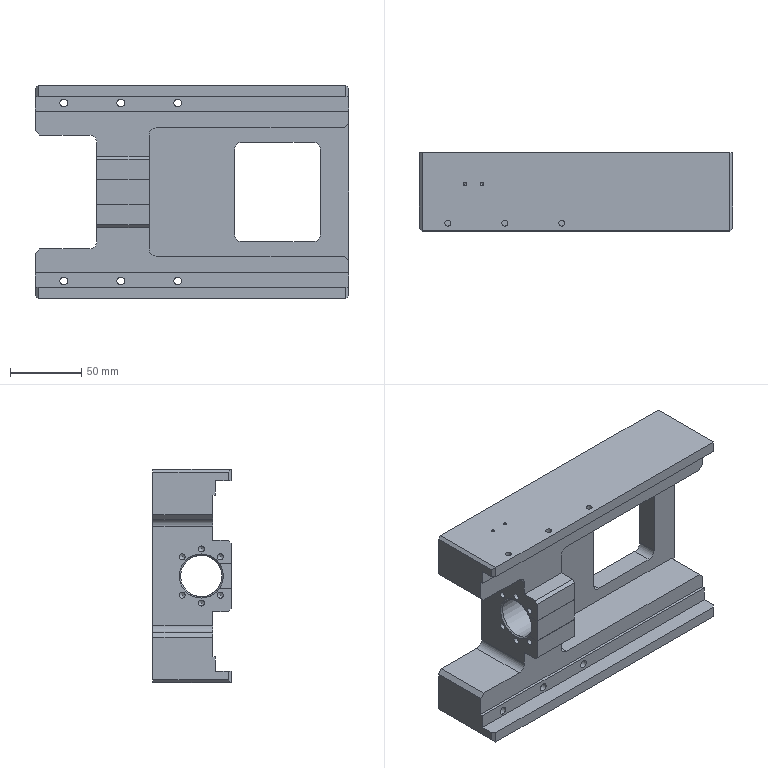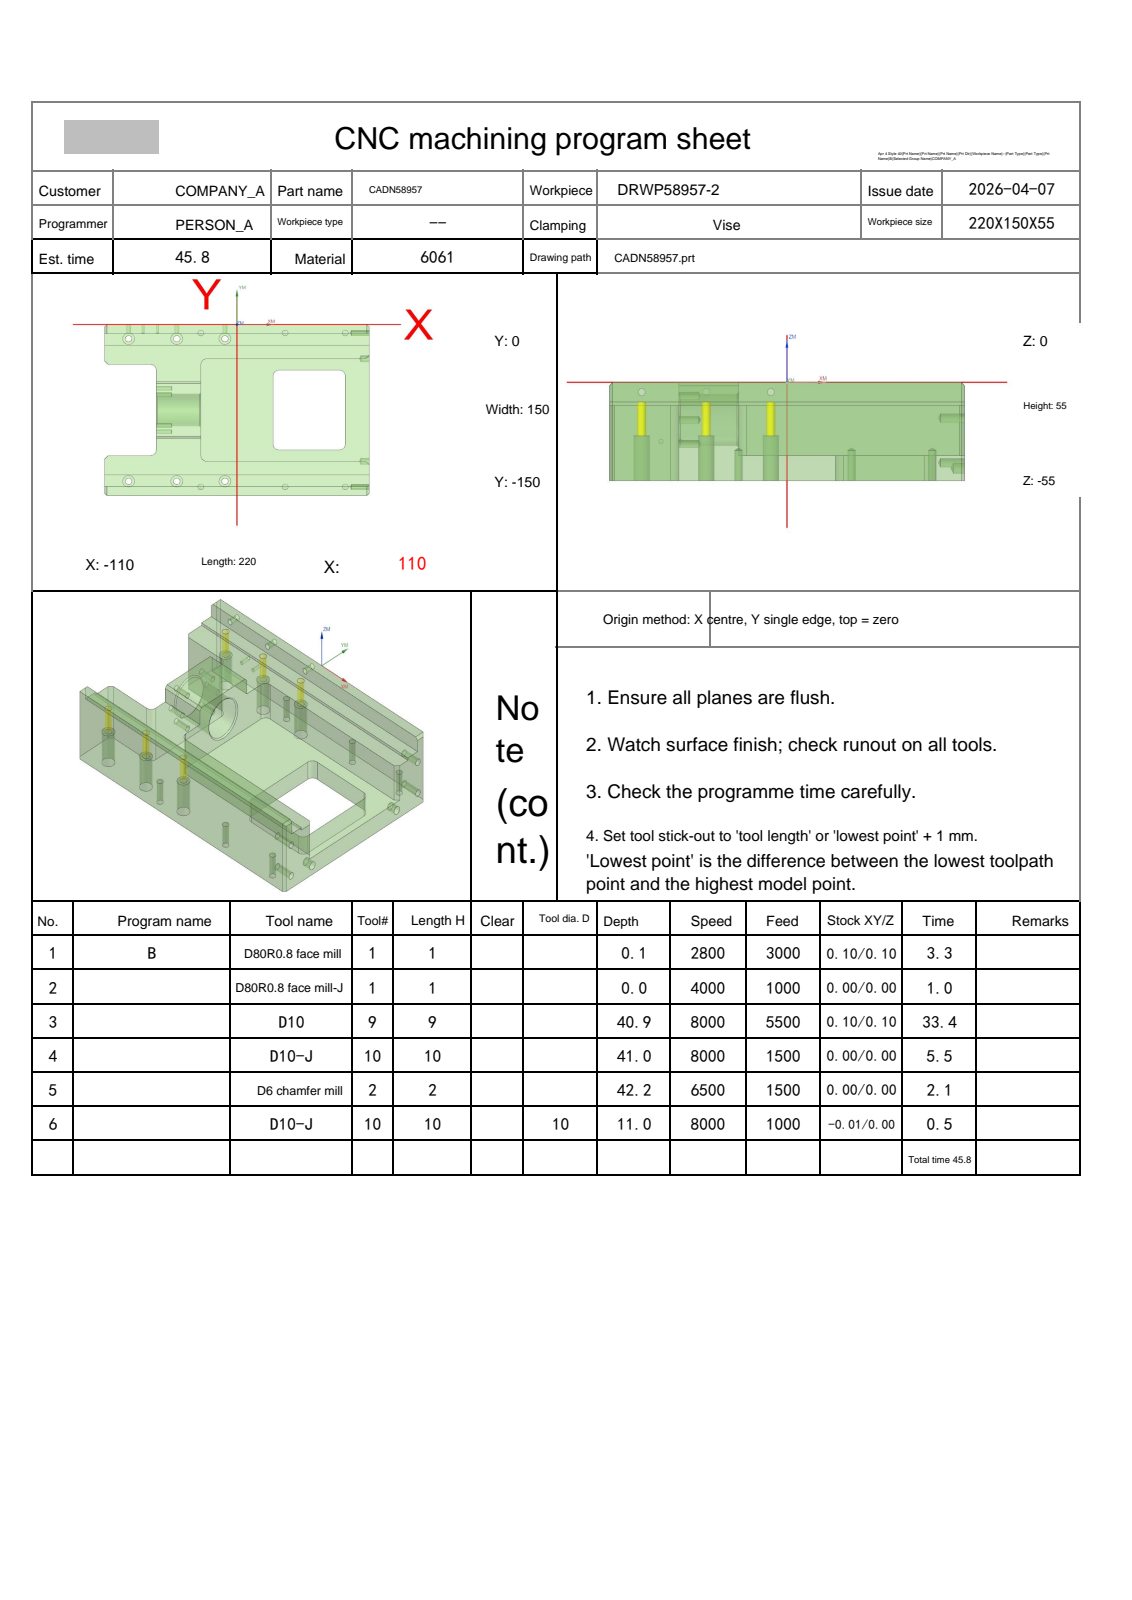NC program | NX | posted by the shop | part box 220 x 55 x 150 mm
Lines 14726 to 15484 of 15484:
N4 T10 M06
(D10-J  D=10. R=0. H=10 ce=0.40 di=0.00)
G00 G90 G54 X-117. Y-128.801 M03 S7000
G43 H10 Z14.5
M08
Z-9.5
G01 Z-11. F1500.
G03 X-115. Y-130.8 I2. J.001
G01 X114.1
G02 X115. Y-131.7 I0.0 J-.9
G01 Y-132.7
G02 X114. Y-133.7 I-1. J0.0
G01 X-114.1
G03 X-115. Y-134.6 I0.0 J-.9
G01 Y-135.6
G03 X-114. Y-136.6 I1. J0.0
G01 X115.
G03 X117. Y-134.6 I0.0 J2.
G01 Z-9.5
G00 Z14.5
Y-124.399
Z-11.5
G01 Z-13.
X113.
G03 X115. Y-126.399 I2. J0.0
G01 X-114.1
G02 X-115. Y-125.499 I0.0 J.9
G01 Y-123.199
G02 X-114. Y-122.199 I1. J0.0
G01 X114.201
G03 X115. Y-121.4 I-.001 J.8
G01 Y-121.343
G03 X114.707 Y-120.636 I-1. J0.0
G01 X112.363 Y-118.292
G03 X111.657 Y-117.999 I-.706 J-.708
G01 X-114.001
G02 X-115. Y-117. I.001 J1.
G01 Y-116.343
G02 X-114.707 Y-115.636 I1. J0.0
G01 X-113.163 Y-114.092
G02 X-112.457 Y-113.8 I.707 J-.708
G01 X-25.9
G03 X-25. Y-112.9 I0.0 J.9
G01 Y-110.6
G03 X-26. Y-109.6 I-1. J0.0
G01 X-71.1
G02 X-72. Y-108.7 I0.0 J.9
G01 Y-106.4
G02 X-71. Y-105.4 I1. J0.0
G01 X-25.
G02 X-23. Y-107.4 I0.0 J-2.
G01 Z-11.5
G00 Z14.5
Y-42.599
Z-11.5
G01 Z-13.
X-27.
G03 X-25. Y-44.599 I2. J0.0
G01 X-71.1
G02 X-72. Y-43.699 I0.0 J.9
G01 Y-41.399
G02 X-71. Y-40.399 I1. J0.0
G01 X-25.9
G03 X-25. Y-39.499 I0.0 J.9
G01 Y-37.199
G03 X-26. Y-36.199 I-1. J0.0
G01 X-112.458
G02 X-113.164 Y-35.907 I.001 J1.
G01 X-114.707 Y-34.364
G02 X-115. Y-33.657 I.707 J.707
G01 Y-32.999
G02 X-114.001 Y-32. I1. J-.001
G01 X111.658
G03 X112.364 Y-31.707 I-.001 J1.
G01 X114.707 Y-29.364
G03 X115. Y-28.657 I-.707 J.707
G01 Y-28.599
G03 X114.201 Y-27.8 I-.8 J-.001
G01 X-114.1
G02 X-115. Y-26.9 I0.0 J.9
G01 Y-24.6
G02 X-114. Y-23.6 I1. J0.0
G01 X115.
G02 X117. Y-25.6 I0.0 J-2.
G01 Z-11.5
G00 Z14.5
Y-21.199
Z-9.5
G01 Z-11.
G03 X115. Y-19.2 I-2. J-.001
G01 X-114.001
G02 X-115. Y-18.201 I.001 J1.
G01 Y-17.299
G02 X-114.001 Y-16.3 I1. J-.001
G01 X114.1
G03 X115. Y-15.4 I0.0 J.9
G01 Y-14.4
G03 X114. Y-13.4 I-1. J0.0
G01 X-115.
G03 X-117. Y-15.4 I0.0 J-2.
G01 Z-9.5
G00 Z14.5
G00 G90 X117. Y-73. M03 S7000
Z14.5
Z-39.5
G01 Z-41. F1500.
X113.
G03 X111. Y-75. I0.0 J-2.
G01 Y-115.882
G02 X110.8 Y-116.08 I-.2 J.001
G01 X110.66 Y-116.023
X109.237 Y-114.6
X-23.603
G02 X-24.6 Y-113.603 I.003 J1.
G01 Y-36.397
G02 X-23.603 Y-35.4 I1. J-.003
G01 X109.237
X110.66 Y-33.977
X110.8 Y-33.92
G02 X111. Y-34.118 I0.0 J-.2
G01 Y-77.086
G02 X110.707 Y-77.793 I-1. J0.0
G01 X106.293 Y-82.207
G03 X106. Y-82.914 I.707 J-.707
G01 Y-108.604
G02 X105.004 Y-109.6 I-1. J.004
G01 X-18.604
G02 X-19.6 Y-108.604 I.004 J1.
G01 Y-41.396
G02 X-18.604 Y-40.4 I1. J-.004
G01 X105.004
G02 X106. Y-41.396 I-.004 J-1.
G01 Y-77.086
G02 X105.707 Y-77.793 I-1. J0.0
G01 X101.293 Y-82.207
G03 X101. Y-82.914 I.707 J-.707
G01 Y-103.604
G02 X100.004 Y-104.6 I-1. J.004
G01 X-13.604
G02 X-14.6 Y-103.604 I.004 J1.
G01 Y-46.396
G02 X-13.604 Y-45.4 I1. J-.004
G01 X100.004
G02 X101. Y-46.396 I-.004 J-1.
G01 Y-77.086
G02 X100.707 Y-77.793 I-1. J0.0
G01 X96.293 Y-82.207
G03 X96. Y-82.914 I.707 J-.707
G01 Y-98.604
G02 X95.004 Y-99.6 I-1. J.004
G01 X-8.604
G02 X-9.6 Y-98.604 I.004 J1.
G01 Y-51.396
G02 X-8.604 Y-50.4 I1. J-.004
G01 X95.004
G02 X96. Y-51.396 I-.004 J-1.
G01 Y-77.086
G02 X95.707 Y-77.793 I-1. J0.0
G01 X91.293 Y-82.207
G03 X91. Y-82.914 I.707 J-.707
G01 Y-93.605
G02 X90.005 Y-94.6 I-1. J.005
G01 X-3.605
G02 X-4.6 Y-93.605 I.005 J1.
G01 Y-56.395
G02 X-3.605 Y-55.4 I1. J-.005
G01 X90.005
G02 X91. Y-56.395 I-.005 J-1.
G01 Y-77.086
G02 X90.707 Y-77.793 I-1. J0.0
G01 X86.293 Y-82.207
G03 X86. Y-82.914 I.707 J-.707
G01 Y-88.605
G02 X85.005 Y-89.6 I-1. J.005
G01 X1.395
G02 X.4 Y-88.605 I.005 J1.
G01 Y-61.395
G02 X1.395 Y-60.4 I1. J-.005
G01 X85.005
G02 X86. Y-61.395 I-.005 J-1.
G01 Y-77.086
G02 X85.707 Y-77.793 I-1. J0.0
G01 X81.292 Y-82.208
G03 X81. Y-82.914 I.708 J-.707
G01 Y-83.605
G02 X80.005 Y-84.6 I-1. J.005
G01 X6.395
G02 X5.4 Y-83.605 I.005 J1.
G01 Y-66.395
G02 X6.395 Y-65.4 I1. J-.005
G01 X80.005
G02 X81. Y-66.395 I-.005 J-1.
G01 Y-76.73
G02 X80.255 Y-77.697 I-1. J0.0
G01 X76.432 Y-78.706
G03 X75.844 Y-79.136 I.256 J-.967
G02 X75.005 Y-79.6 I-.844 J.536
G01 X11.395
G02 X10.4 Y-78.605 I.005 J1.
G01 Y-71.395
G02 X11.395 Y-70.4 I1. J-.005
G01 X75.005
G02 X76. Y-71.395 I-.005 J-1.
G01 Y-78.605
G02 X75.974 Y-78.827 I-1. J.005
X75.335 Y-79.542 I-.974 J.227
G03 X74.005 Y-81.427 I.67 J-1.884
X74.12 Y-82.097 I2. J0.0
G01 Z-39.5
G00 Z14.5
G00 G90 X117. Y-25.399 M03 S8000
Z14.5
Z-12.
G01 Z-13. F1000.
G41 D10
Y-25.199
G03 X115. Y-23.2 I-2. J-.001
G01 X-115.
G03 X-117. Y-25.199 I0.0 J-2.
G01 G40 Y-25.399
Z-12.
G00 X-74. Y-42.801
G01 Z-13.
G41 D10
Y-43.001
G03 X-72. Y-45. I2. J.001
G01 X-25.
G03 X-23. Y-43.001 I0.0 J2.
G01 G40 Y-42.801
Z-12.
G00 Z3.
Y-107.199
Z-12.
G01 Z-13.
G41 D10
Y-106.999
G03 X-25. Y-105. I-2. J-.001
G01 X-72.
G03 X-74. Y-106.999 I0.0 J-2.
G01 G40 Y-107.199
Z-12.
G00 X-117. Y-124.601
G01 Z-13.
G41 D10
Y-124.801
G03 X-115. Y-126.8 I2. J.001
G01 X115.
G03 X117. Y-124.801 I0.0 J2.
G01 G40 Y-124.601
Z-12.
G00 Z14.5
G00 G90 X117.191 Y-28.632 M03 S8000
Z14.5
Z-12.667
G01 Z-13.667 F1000.
G41 D10
X117. Y-28.573
G03 X116.414 Y-28.485 I-.586 J-1.912
X115. Y-29.071 I0.0 J-2.
G01 X109.071 Y-35.
X-25.
Y-115.
X109.071
X115. Y-120.929
G03 X116.414 Y-121.515 I1.414 J1.414
X117. Y-121.427 I0.0 J2.
G01 G40 X117.191 Y-121.368
Z-12.667
G00 Y-28.632
Z-26.333
G01 Z-27.333
G41 D10
X117. Y-28.573
G03 X116.414 Y-28.485 I-.586 J-1.912
X115. Y-29.071 I0.0 J-2.
G01 X109.071 Y-35.
X-25.
Y-115.
X109.071
X115. Y-120.929
G03 X116.414 Y-121.515 I1.414 J1.414
X117. Y-121.427 I0.0 J2.
G01 G40 X117.191 Y-121.368
Z-26.333
G00 Y-28.632
Z-40.
G01 Z-41.
G41 D10
X117. Y-28.573
G03 X116.414 Y-28.485 I-.586 J-1.912
X115. Y-29.071 I0.0 J-2.
G01 X109.071 Y-35.
X-25.
Y-115.
X109.071
X115. Y-120.929
G03 X116.414 Y-121.515 I1.414 J1.414
X117. Y-121.427 I0.0 J2.
G01 G40 X117.191 Y-121.368
Z-40.
G00 Z14.5
G91 G28 Z0.0
M05
M09
G91 G28 Z0.0
M01
N5 T02 M06
(D6 chamfer mill  D=6. R=0. H=02 ce=0.00 di=0.00)
G00 G90 G54 X-108.792 Y-141.01 M03 S6500
G43 H02 Z20.
M08
Z.13
G01 Z-1.2 F1500.
G03 X-108.452 Y-141.085 I.601 J1.907
G01 X-108.398 Y-141.095
X-108.349 Y-141.072
X-108.259 Y-141.034
X-108. Y-141.
X108.
X108.259 Y-141.034
X108.349 Y-141.072
X108.398 Y-141.095
X108.452 Y-141.085
G03 X108.792 Y-141.01 I-.261 J1.983
G01 Z.13
G00 Z2.8
X108.903 Y-150.41
G01 Z-1.2
X108.866 Y-150.5
X108.707 Y-150.707
X108.5 Y-150.866
X108.259 Y-150.966
X108. Y-151.
X0.0
X-108.
X-108.259 Y-150.966
X-108.5 Y-150.866
X-108.707 Y-150.707
X-108.866 Y-150.5
X-108.903 Y-150.41
Z2.8
G00 Z10.
X-67.99 Y-98.792
Z.13
G01 Z-1.2
G03 X-67.915 Y-98.452 I-1.907 J.601
G01 X-67.905 Y-98.398
X-67.928 Y-98.349
X-67.966 Y-98.259
X-68. Y-98.
Y-52.
X-67.966 Y-51.741
X-67.928 Y-51.651
X-67.905 Y-51.602
X-67.915 Y-51.548
G03 X-67.99 Y-51.208 I-1.983 J-.261
G01 Z.13
G00 Z10.
X-29.01
Z.13
G01 Z-1.2
G03 X-29.085 Y-51.548 I1.907 J-.601
G01 X-29.095 Y-51.602
X-29.072 Y-51.651
X-29.034 Y-51.741
X-29. Y-52.
Y-75.
Y-98.
X-29.034 Y-98.259
X-29.072 Y-98.349
X-29.095 Y-98.398
X-29.085 Y-98.452
G03 X-29.01 Y-98.792 I1.983 J.261
G01 Z.13
G00 Z10.
X-108.903 Y.41
Z2.8
G01 Z-1.2
X-108.866 Y.5
X-108.707 Y.707
X-108.5 Y.866
X-108.259 Y.966
X-108. Y1.
X108.
X108.259 Y.966
X108.5 Y.866
X108.707 Y.707
X108.866 Y.5
X108.903 Y.41
Z2.8
G00 X108.792 Y-8.99
Z.13
G01 Z-1.2
G03 X108.452 Y-8.915 I-.601 J-1.907
G01 X108.398 Y-8.905
X108.349 Y-8.928
X108.259 Y-8.966
X108. Y-9.
X0.0
X-108.
X-108.259 Y-8.966
X-108.349 Y-8.928
X-108.398 Y-8.905
X-108.452 Y-8.915
G03 X-108.792 Y-8.99 I.261 J-1.983
G01 Z.13
G00 Z10.
X111.068 Y-11.032
Z-2.305
G01 Z-12.2
X111.008 Y-11.118
X111. Y-11.148
Y-18.2
G02 X110. Y-19.2 I-1. J0.0
G01 X-110.
G02 X-111. Y-18.2 I0.0 J1.
G01 Y-11.118
X-111.005 Y-11.098
X-111.045 Y-11.041
Z-2.292
G00 Z10.
X-10.828 Y-11.209
Z-1.81
G01 Z-12.2
G03 X-11.174 Y-11.251 I.07 J-1.999
G01 X-11.228 Y-11.26
X-11.267 Y-11.298
X-11.301 Y-11.329
G03 X-11.75 Y-12.5 I1.301 J-1.171
X-10. Y-14.25 I1.75 J0.0
X-8.25 Y-12.5 I0.0 J1.75
X-8.336 Y-11.959 I-1.75 J0.0
G01 X-8.484 Y-11.625
X-8.699 Y-11.329
X-8.733 Y-11.298
X-8.768 Y-11.274
X-8.811 Y-11.24
X-8.865 Y-11.237
X-9.06 Y-11.228
X-9.214 Y-11.234
Z-1.835
G00 Z10.
X-50.828 Y-11.209
Z-1.81
G01 Z-12.2
G03 X-51.174 Y-11.251 I.07 J-1.999
G01 X-51.228 Y-11.26
X-51.267 Y-11.298
X-51.301 Y-11.329
G03 X-51.75 Y-12.5 I1.301 J-1.171
X-50. Y-14.25 I1.75 J0.0
X-48.25 Y-12.5 I0.0 J1.75
X-48.336 Y-11.959 I-1.75 J0.0
G01 X-48.484 Y-11.625
X-48.699 Y-11.329
X-48.733 Y-11.298
X-48.768 Y-11.274
X-48.811 Y-11.24
X-48.865 Y-11.237
X-49.06 Y-11.228
X-49.214 Y-11.234
Z-1.835
G00 Z10.
X-90.828 Y-11.209
Z-1.81
G01 Z-12.2
G03 X-91.174 Y-11.251 I.07 J-1.999
G01 X-91.228 Y-11.26
X-91.267 Y-11.298
X-91.301 Y-11.329
G03 X-91.75 Y-12.5 I1.301 J-1.171
X-90. Y-14.25 I1.75 J0.0
X-88.25 Y-12.5 I0.0 J1.75
X-88.336 Y-11.959 I-1.75 J0.0
G01 X-88.484 Y-11.625
X-88.699 Y-11.329
X-88.733 Y-11.298
X-88.768 Y-11.274
X-88.811 Y-11.24
X-88.865 Y-11.237
X-89.06 Y-11.228
X-89.214 Y-11.234
Z-1.835
G00 Z10.
X-111.068 Y-138.968
Z-2.305
G01 Z-12.2
X-111.008 Y-138.882
X-111. Y-138.852
Y-131.8
G02 X-110. Y-130.8 I1. J0.0
G01 X110.
G02 X111. Y-131.8 I0.0 J-1.
G01 Y-138.882
X111.005 Y-138.902
X111.045 Y-138.959
Z-2.292
G00 Z10.
X-9.172 Y-138.791
Z-1.81
G01 Z-12.2
G03 X-8.826 Y-138.749 I-.07 J1.999
G01 X-8.772 Y-138.74
X-8.733 Y-138.702
X-8.699 Y-138.671
G03 X-8.25 Y-137.5 I-1.301 J1.171
X-10. Y-135.75 I-1.75 J0.0
X-11.75 Y-137.5 I0.0 J-1.75
X-11.664 Y-138.041 I1.75 J0.0
G01 X-11.516 Y-138.375
X-11.301 Y-138.671
X-11.267 Y-138.702
X-11.232 Y-138.726
X-11.189 Y-138.76
X-11.135 Y-138.763
X-10.94 Y-138.772
X-10.786 Y-138.766
Z-1.835
G00 Z10.
X-49.172 Y-138.791
Z-1.81
G01 Z-12.2
G03 X-48.826 Y-138.749 I-.07 J1.999
G01 X-48.772 Y-138.74
X-48.733 Y-138.702
X-48.699 Y-138.671
G03 X-48.25 Y-137.5 I-1.301 J1.171
X-50. Y-135.75 I-1.75 J0.0
X-51.75 Y-137.5 I0.0 J-1.75
X-51.664 Y-138.041 I1.75 J0.0
G01 X-51.516 Y-138.375
X-51.301 Y-138.671
X-51.267 Y-138.702
X-51.232 Y-138.726
X-51.189 Y-138.76
X-51.135 Y-138.763
X-50.94 Y-138.772
X-50.786 Y-138.766
Z-1.835
G00 Z10.
X-89.172 Y-138.791
Z-1.81
G01 Z-12.2
G03 X-88.826 Y-138.749 I-.07 J1.999
G01 X-88.772 Y-138.74
X-88.733 Y-138.702
X-88.699 Y-138.671
G03 X-88.25 Y-137.5 I-1.301 J1.171
X-89.636 Y-135.788 I-1.75 J0.0
G01 X-90. Y-135.75
G03 X-91.75 Y-137.5 I0.0 J-1.75
X-91.516 Y-138.375 I1.75 J0.0
G01 X-91.301 Y-138.671
X-91.267 Y-138.702
X-91.232 Y-138.726
X-91.189 Y-138.76
X-91.135 Y-138.763
X-90.94 Y-138.772
X-90.786 Y-138.766
Z-1.835
G00 Z10.
X-68.068 Y-46.991
Z-3.086
G01 Z-14.2
X-68.008 Y-46.905
X-68. Y-46.875
Y-40.
G03 X-72. Y-36. I-4. J0.0
G01 X-107.
X-107.259 Y-35.966
X-107.5 Y-35.866
X-107.707 Y-35.707
X-110.707 Y-32.707
X-110.866 Y-32.5
X-110.966 Y-32.259
X-111. Y-32.
Y-21.3
X-111.008 Y-21.27
X-111.068 Y-21.184
Z-12.669
G00 Z10.
X111.068 Y-21.178
Z-12.669
G01 Z-14.2
X111.008 Y-21.264
X111. Y-21.294
Y-27.
X110.966 Y-27.259
X110.866 Y-27.5
X110.707 Y-27.707
X107.707 Y-30.707
X107.5 Y-30.866
X107.259 Y-30.966
X107. Y-31.
X-25.
G03 X-29. Y-35. I0.0 J-4.
G01 Y-46.865
X-28.992 Y-46.895
X-28.932 Y-46.981
Z-3.096
G00 Z10.
X-111.068 Y-128.816
Z-12.669
G01 Z-14.2
X-111.008 Y-128.73
X-111. Y-128.7
Y-118.
X-110.966 Y-117.741
X-110.866 Y-117.5
X-110.707 Y-117.293
X-107.707 Y-114.293
X-107.5 Y-114.134
X-107.259 Y-114.034
X-107. Y-114.
X-72.
G03 X-68. Y-110. I0.0 J4.
G01 Y-103.125
X-68.008 Y-103.095
X-68.068 Y-103.009
Z-3.086
G00 Z10.
X-28.932 Y-103.019
Z-3.096
G01 Z-14.2
X-28.992 Y-103.105
X-29. Y-103.135
Y-115.
G03 X-25. Y-119. I4. J0.0
G01 X107.
X107.259 Y-119.034
X107.5 Y-119.134
X107.707 Y-119.293
X110.707 Y-122.293
X110.866 Y-122.5
X110.966 Y-122.741
X111. Y-123.
Y-128.706
X111.008 Y-128.736
X111.068 Y-128.822
Z-12.669
G00 Z10.
X111.204 Y-30.309
Z-14.793
G01 Z-42.199
G03 X111.024 Y-30.566 I1.379 J-1.157
G01 X110.996 Y-30.607
X111. Y-30.656
Y-119.344
X110.996 Y-119.393
X111.024 Y-119.434
G03 X111.204 Y-119.691 I1.559 J.9
G01 Z-14.793
G00 Z10.
X31.227 Y-74.614
Z-40.828
G01 Z-42.199
G03 X31.027 Y-74.9 I1.532 J-1.286
G01 X30.997 Y-74.946
X31. Y-75.
Y-105.
G03 X35. Y-109. I4. J0.0
G01 X85.
G03 X89. Y-105. I0.0 J4.
G01 Y-45.
G03 X85. Y-41. I-4. J0.0
G01 X35.
G03 X31. Y-45. I0.0 J-4.
G01 Y-75.
X30.997 Y-75.054
X31.027 Y-75.1
G03 X31.227 Y-75.386 I1.732 J1.
G01 Z-40.828
G00 Z20.
G00 G90 X-111.516 Y-11.9 M03 S6500
Z20.
Z-1.2
G01 Z-2.7 F1500.
G03 X-110.7 Y-10.763 I-.384 J1.137
G01 Y1.207
G03 X-111.9 Y2.407 I-1.2 J0.0
G01 Z-1.2
G00 Z20.
X-70.9 Y-48.484
Z-1.2
G01 Z-2.7
G03 X-69.763 Y-49.3 I1.137 J.384
G01 X-27.237
G03 X-26.1 Y-48.484 I0.0 J1.2
G01 Z-1.2
G00 Z20.
Y-101.516
Z-1.2
G01 Z-2.7
G03 X-27.237 Y-100.7 I-1.137 J-.384
G01 X-69.763
G03 X-70.9 Y-101.516 I0.0 J-1.2
G01 Z-1.2
G00 Z20.
X-111.9 Y-152.407
Z-1.2
G01 Z-2.7
G03 X-110.7 Y-151.207 I0.0 J1.2
G01 Y-139.237
G03 X-111.516 Y-138.1 I-1.2 J0.0
G01 Z-1.2
G00 Z20.
X111.516
Z-1.2
G01 Z-2.7
G03 X110.7 Y-139.237 I.384 J-1.137
G01 Y-151.207
G03 X111.9 Y-152.407 I1.2 J0.0
G01 Z-1.2
G00 Z20.
Y2.407
Z-1.2
G01 Z-2.7
G03 X110.7 Y1.207 I0.0 J-1.2
G01 Y-10.763
G03 X111.516 Y-11.9 I1.2 J0.0
G01 Z-1.2
G00 Z20.
G91 G28 Z0.0
M05
M09
G91 G28 Z0.0
M01
N6 T10 M06
(D10-J  D=10. R=0. H=10 ce=-0.01 di=0.00)
G00 G90 G54 X117.01 Y-14.989 M03 S8000
G43 H10 Z14.5
M08
Z-10.
G01 Z-11. F1000.
G41 D10
X116.99 Y-14.79
G03 X115. Y-12.99 I-1.99 J-.2
G01 X-115.
G03 X-116.99 Y-14.79 I0.0 J-2.
G01 G40 X-117.01 Y-14.989
Z-10.
G00 Z3.
Y-135.011
Z-10.
G01 Z-11.
G41 D10
X-116.99 Y-135.21
G03 X-115. Y-137.01 I1.99 J.2
G01 X115.
G03 X116.99 Y-135.21 I0.0 J2.
G01 G40 X117.01 Y-135.011
Z-10.
G00 Z14.5
M05
M09
G91 G28 Z0.0
G91 G28 Y0.0
M30
%